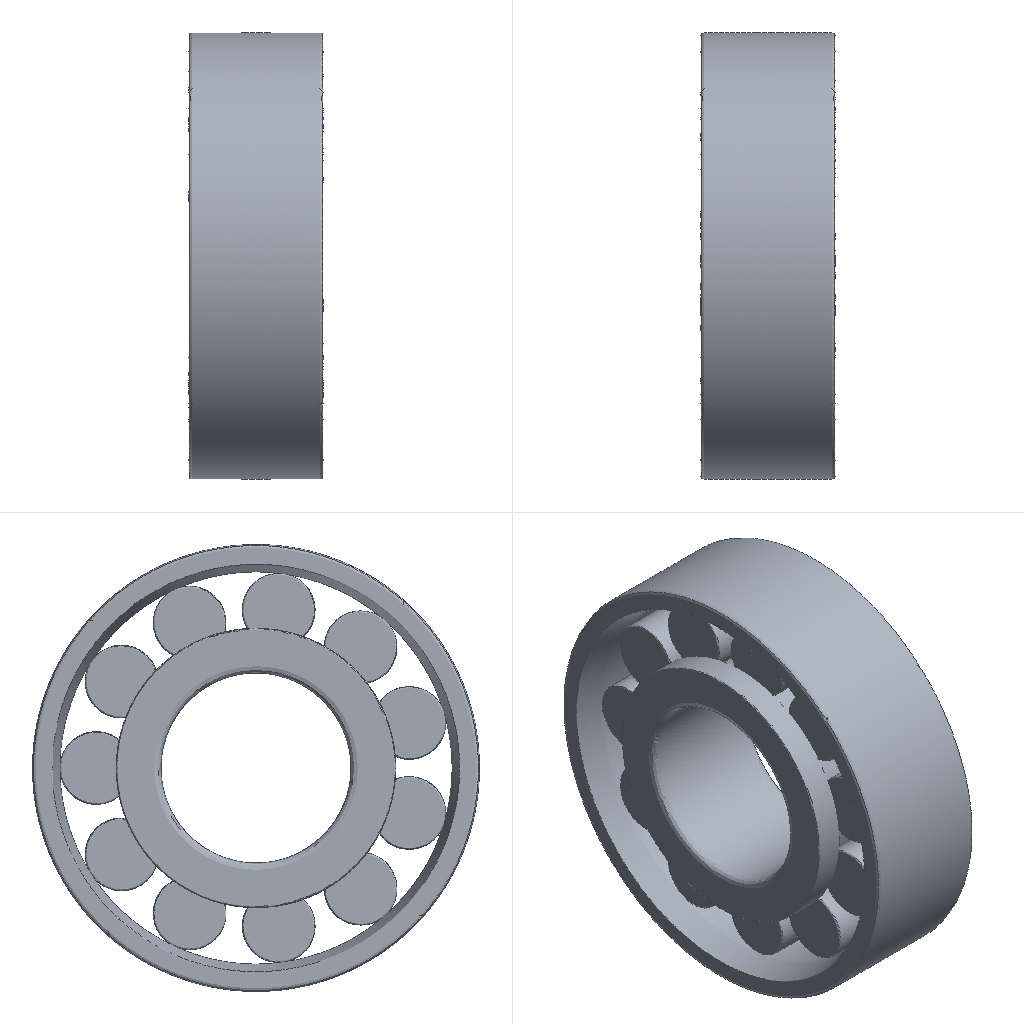Simulation study | ansys workbench
Set-up summary:
category,name,step,type,value,unit,region
solver,ansys_workbench
units,mm-N-s-tonne (MPa),,stated,"/units,MPA"
analysis,LS1,,static
load_step,LS1,LS1,static,nsubst=1; time=1
mesh,nodes,,,877286
mesh,elements,,,641316
element_type,SOLID187,,,594392
element_type,TARGE170,,,16923
element_type,CONTA174,,,16923
element_type,SURF154,,,13078
material,Structural Steel,,E,200000,tonne s^-2 mm^-1
material,Structural Steel,,nu,0.3
material,Structural Steel,,density,7.85e-09,tonne mm^-3
material,Structural Steel,,conductivity,60.5,tonne mm s^-3 C^-1
material,Structural Steel,,specific_heat,4.34e+08,mm^2 s^-2 C^-1
material,Structural Steel,,cte,1.2e-05,C^-1
material,Structural Steel,,permeability,10000
material,Structural Steel,,resistivity,0.00017,ohm mm
load,Define Force Using Surface Effect Elements,LS1,surface-effect pres face 2,-0.349,,SURF154 #8
bc,Constant Zero Displacement X,model,fixed,[dofs=UX],,_DISPZEROUX
bc,Constant Zero Displacement Y,model,fixed,[dofs=UY],,_DISPZEROUY
bc,Constant Zero Displacement Z,model,fixed,[dofs=UZ],,_DISPZEROUZ
contact,Contact Region,,bonded (always),element=CONTA174
contact,Contact Region 2,,bonded (always),element=CONTA174
named_set,_DISPZEROUX,,node,26660
named_set,_DISPZEROUY,,node,26660
named_set,_DISPZEROUZ,,node,26660
Ansys APDL input file, long lists of numbers shortened:
/batch
/config,noeldb,1     ! force off writing results to database
*get,_wallstrt,active,,time,wall
! ANSYS input file written by Workbench version 2022 R2
! File used for geometry attach:
/title,____--____ (A5)
! ****** Begin Custom Load Command Snippet ******
/COM, ACT Extensions:
/COM,     LSDYNA, 2022.2
/COM,/COM,     ANSYSMotion, 2022.2
/COM,
! ****** End   Custom Load Command Snippet ******
*DIM,_wb_ProjectScratch_dir,string,248
_wb_ProjectScratch_dir(1) = ''
*DIM,_wb_SolverFiles_dir,string,248
_wb_SolverFiles_dir(1) = ''
*DIM,_wb_userfiles_dir,string,248
_wb_userfiles_dir(1) = ''
/com,--- Data in consistent NMM units. See Solving Units in the help system for more information.
/units,MPA
/nopr
/wb,file,start              !  signify a WB generated input file
/prep7
! Turn off shape checking because checks already performed inside WB mesher.
! See help system for more information.
SHPP,OFF,,NOWARN
/nolist
etcon,set             ! allow ANSYS to choose best KEYOP's for 180x elements, resets any applicable keyopt to MAPDL defaults
/com,*********** Nodes for the whole assembly ***********
nblock,3,,965014
(1i9,3e20.9e3)
        1     6.000000000E-01     8.500000000E+00     0.000000000E+00
! (877285 more lines like these left out)
-1
/wb,elem,start            !  set before creation of elements
/com,*********** Elements for Body 1 "skf_bearing_n_203_ecp_2_1" ***********
et,1,187
eblock,19,solid,,168754
(19i9)
        1        1        1        1        0        0        0        0       10        0        1    24241    33706    28817    28794   205578   234077   205576   205574
! (337507 more lines like these left out)
-1
/com,*********** Elements for Body 2 "skf_bearing_n_203_ecp_2_2" ***********
et,2,187
eblock,19,solid,,244984
(19i9)
        2        2        2        2        0        0        0        0       10        0   349409   532471   543456   562473   549157   703456   779981   703461   703457
! (489967 more lines like these left out)
-1
/com,*********** Elements for Body 3 "skf_bearing_n_203_ecp_2_3" ***********
et,3,187
eblock,19,solid,,180654
(19i9)
        3        3        3        3        0        0        0        0       10        0   168755   276452   283271   278432   279668   480271   491944   480267   480268
! (361307 more lines like these left out)
-1
/wb,elem,end               !  done creating elements
/com,*********** Send User Defined Coordinate System(s) ***********
csys,0
toffst,273.15,  ! Temperature offset from absolute zero
/com,*********** Set Reference Temperature ***********
tref,22.
/wb,mat,start              !  starting to send materials
/com,*********** Send Materials ***********
Temperature = 'TEMP' ! Temperature
MP,DENS,1,7.85e-09,	! tonne mm^-3
MP,ALPX,1,1.2e-05,	! C^-1
MP,C,1,434000000,	! mm^2 s^-2 C^-1
MP,KXX,1,60.5,	! tonne mm s^-3 C^-1
MP,RSVX,1,0.00017,	! ohm mm
MP,EX,1,200000,	! tonne s^-2 mm^-1
MP,NUXY,1,0.3,
MP,MURX,1,10000,
Temperature = 'TEMP' ! Temperature
MP,DENS,2,7.85e-09,	! tonne mm^-3
MP,ALPX,2,1.2e-05,	! C^-1
MP,C,2,434000000,	! mm^2 s^-2 C^-1
MP,KXX,2,60.5,	! tonne mm s^-3 C^-1
MP,RSVX,2,0.00017,	! ohm mm
MP,EX,2,200000,	! tonne s^-2 mm^-1
MP,NUXY,2,0.3,
MP,MURX,2,10000,
Temperature = 'TEMP' ! Temperature
MP,DENS,3,7.85e-09,	! tonne mm^-3
MP,ALPX,3,1.2e-05,	! C^-1
MP,C,3,434000000,	! mm^2 s^-2 C^-1
MP,KXX,3,60.5,	! tonne mm s^-3 C^-1
MP,RSVX,3,0.00017,	! ohm mm
MP,EX,3,200000,	! tonne s^-2 mm^-1
MP,NUXY,3,0.3,
MP,MURX,3,10000,
/wb,mat,end                !  done sending materials
!************************* Model Summary ********************
!skf_bearing_n_203_ecp_2_1,	结构钢,	matid,	1
!skf_bearing_n_203_ecp_2_2,	结构钢,	matid,	2
!skf_bearing_n_203_ecp_2_3,	结构钢,	matid,	3
!************************* End Model Summary ********************
! get the diagonal of the bounding box. Needed later for other things
*get,_xmin,node,,mnloc,x
*get,_ymin,node,,mnloc,y
*get,_zmin,node,,mnloc,z
*get,_xmax,node,,mxloc,x
*get,_ymax,node,,mxloc,y
*get,_zmax,node,,mxloc,z
_ASMDIAG=(_xmax-_xmin)*(_xmax-_xmin)+(_ymax-_ymin)*(_ymax-_ymin)+(_zmax-_zmin)*(_zmax-_zmin)
_ASMDIAG=SQRT(_ASMDIAG)
/wb,contact,start          !  starting to send contact
/com,*********** Create Contact "接触区域" ***********
/com,            Real Constant Set For Above Contact Is 5 & 4
*set,tid,5
*set,cid,4
r,tid
r,cid
et,tid,170
et,cid,174
eblock,10,,,4315
(15i9)
   675971        5        5        5        0     8715     8859     8791     8791    93916    94399     8791    93915
! (4314 more lines like these left out)
-1
eblock,10,,,4315
(15i9)
   680286        4        4        4        0     8715     8859     8791     8791    93916    94399     8791    93915
! (4314 more lines like these left out)
-1
eblock,10,,,5558
(15i9)
   684601        4        5        4        0   258107   258138   258199   258199   357645   357931   258199   357648
! (5557 more lines like these left out)
-1
eblock,10,,,5558
(15i9)
   690159        5        4        5        0   258107   258138   258199   258199   357645   357931   258199   357648
! (5557 more lines like these left out)
-1
keyo,cid,8,2               ! auto create asymmetric contact (from Program Controlled setting)
keyo,cid,10,0              ! adjust contact stiffness each NR iteration (from Program Controlled setting)
keyo,cid,12,5              ! bonded always
keyo,cid,18,1              ! small sliding turned on by application
keyo,cid,2,0               ! augmented Lagrange (from Program Controlled setting)
keyo,cid,4,0               ! on Gauss point (from Program Controlled setting)
keyo,cid,9,1               ! ignore initial gaps/penetration
keyo,cid,7,0               ! No Prediction
rmod,tid,3,10.      ! FKN
rmod,tid,5,0.       ! ICONT
rmod,tid,6,0.       ! PINB
rmod,tid,10,0.      ! CNOF
rmod,tid,12,0.      ! FKT
rmod,tid,36,32      ! WB DSID
rmod,cid,3,10.      ! FKN
rmod,cid,5,0.       ! ICONT
rmod,cid,6,0.       ! PINB
rmod,cid,10,0.      ! CNOF
rmod,cid,12,0.      ! FKT
rmod,cid,36,32      ! WB DSID
/com,*********** Create Contact "接触区域 2" ***********
/com,            Real Constant Set For Above Contact Is 7 & 6
*set,tid,7
*set,cid,6
r,tid
r,cid
et,tid,170
et,cid,174
eblock,10,,,3223
(15i9)
   695717        7        7        7        0   512910   513130   519477   519477   571635   573570   519477   571638
! (3222 more lines like these left out)
-1
eblock,10,,,3223
(15i9)
   698940        6        6        6        0   512910   513130   519477   519477   571635   573570   519477   571638
! (3222 more lines like these left out)
-1
eblock,10,,,3827
(15i9)
   702163        6        7        6        0   246843   246842   249430   249430   283277   283280   249430   283288
! (3826 more lines like these left out)
-1
eblock,10,,,3827
(15i9)
   705990        7        6        7        0   246843   246842   249430   249430   283277   283280   249430   283288
! (3826 more lines like these left out)
-1
keyo,cid,8,2               ! auto create asymmetric contact (from Program Controlled setting)
keyo,cid,10,0              ! adjust contact stiffness each NR iteration (from Program Controlled setting)
keyo,cid,12,5              ! bonded always
keyo,cid,18,1              ! small sliding turned on by application
keyo,cid,2,0               ! augmented Lagrange (from Program Controlled setting)
keyo,cid,4,0               ! on Gauss point (from Program Controlled setting)
keyo,cid,9,1               ! ignore initial gaps/penetration
keyo,cid,7,0               ! No Prediction
rmod,tid,3,10.      ! FKN
rmod,tid,5,0.       ! ICONT
rmod,tid,6,0.       ! PINB
rmod,tid,10,0.      ! CNOF
rmod,tid,12,0.      ! FKT
rmod,tid,36,35      ! WB DSID
rmod,cid,3,10.      ! FKN
rmod,cid,5,0.       ! ICONT
rmod,cid,6,0.       ! PINB
rmod,cid,10,0.      ! CNOF
rmod,cid,12,0.      ! FKT
rmod,cid,36,35      ! WB DSID
nsel,all
esel,all
/wb,contact,end            !  done creating contacts
/golist
/wb,load,start             !  starting to send loads
/com,******* Constant Zero Displacement X *******
CMBLOCK,_DISPZEROUX,NODE,    26660
(8i10)
    511700    511701    511702    511703    511704    511705    511706    511707
! (3332 more lines like these left out)
cmsel,s,_DISPZEROUX
d,all,ux,0
nsel,all
/com,******* Constant Zero Displacement Y *******
CMBLOCK,_DISPZEROUY,NODE,    26660
(8i10)
    511700    511701    511702    511703    511704    511705    511706    511707
! (3332 more lines like these left out)
cmsel,s,_DISPZEROUY
d,all,uy,0
nsel,all
/com,******* Constant Zero Displacement Z *******
CMBLOCK,_DISPZEROUZ,NODE,    26660
(8i10)
    511700    511701    511702    511703    511704    511705    511706    511707
! (3332 more lines like these left out)
cmsel,s,_DISPZEROUZ
d,all,uz,0
nsel,all
/com,*********** Define Force Using Surface Effect Elements ***********
local,12,0,0.,0.,0.,0.,0.,0.
csys,0
et,8,154
eblock,10,,,13078
(15i9)
   709817        8        8        8       12   511959   511958   522804   522804   564554   564557   522804   564565
! (13077 more lines like these left out)
-1
esel,s,type,,8
keyop,8,2,1                ! Apply load in local coordinate system
keyop,8,7,1                ! Use original area so load is constant in large deformation
esel,all
/com,*********** Define Rotational Velocity ***********
esel,none
esel,a,type,,1
cm,cm_rotvelcity50,elem
esel,all
/gst,on,on
fini
*get,_numnode,node,0,count
*get,_numelem,elem,0,count
*get, _MAXELEMNUM, elem, 0, NUM, MAX
*get, _MAXNODENUM, node, 0, NUM, MAX
*get, _MAXELEMTYPE, etyp, 0, NUM, MAX
*get, _MAXREALCONST, rcon, 0, NUM, MAX
/go
/wb,load,end               !  done creating loads
/com,--- Number of total nodes = %_numnode%
/com,--- Number of contact elements = 46924
/com,--- Number of spring elements = 0
/com,--- Number of bearing elements = 0
/com,--- Number of solid elements = 594392
/com,--- Number of condensed parts = 0
/com,--- Number of total elements = %_numelem%
*get,_wallbsol,active,,time,wall
/com,****************************************************************************
/com,*************************    SOLUTION       ********************************
/com,****************************************************************************
/solu
antype,0                   ! static analysis
_thickRatio=  1     ! Ratio of thick parts in the model
eqsl,pcg,1e-8,,,,,,1
cntr,print,1               ! print out contact info and also make no initial contact an error
dmpoption,emat,no             ! Don't combine emat file for DANSYS
dmpoption,esav,no             ! Don't combine esav file for DANSYS
nldiag,cont,iter           ! print out contact info each equilibrium iteration
rescontrol,,none                 ! Do not keep any restart files
/com,****************************************************
/com,******************* SOLVE FOR LS 1 OF 1 ****************
esel,s,type,,8
nsle
sfe,all,1,pres,1,0.
sfe,all,2,pres,1,-0.349
sfe,all,3,pres,1,0.
nsel,all
esel,all
cmom,cm_rotvelcity50,200.,0.,0.,6.,0.,0.
/nopr
/gopr
nsub,1,1,1
time,1.
outres,erase
outres,all,none
outres,nsol,all,
outres,rsol,all
outres,eangl,all
outres,etmp,all
outres,veng,all
outres,strs,all,
outres,epel,all,
outres,eppl,all,
outres,cont,all,
! *********** WB SOLVE COMMAND ***********
! check interactive state
*get,ANSINTER_,active,,int
*if,ANSINTER_,ne,0,then
/eof
*endif
solve
/com *************** Write FE CONNECTORS *********
CEWRITE,file,ce,,INTE
/com,****************************************************
/com,*************** FINISHED SOLVE FOR LS 1 *************
*get,_wallasol,active,,time,wall
/nopr
*get,_numnode,node,0,count
*get,_numelem,elem,0,count
*get, _MAXELEMNUM, elem, 0, NUM, MAX
*get, _MAXNODENUM, node, 0, NUM, MAX,,,INTERNAL
*get, _MAXELEMTYPE, etyp, 0, NUM, MAX
*get, _MAXREALCONST, rcon, 0, NUM, MAX
*get,_NSOLTHREADS,active,0,ntfs
*get,_NSOLPROCESSES,active,0,npfs
/gopr
*get,_PCGITER,active,,solu,cgiter
/post1
xmlo,ENCODING,ISO-8859-1
xmlo,parm
/xml,parm,xml
fini
/gopr
*get,_walldone,active,,time,wall
_preptime=(_wallbsol-_wallstrt)*3600
_solvtime=(_wallasol-_wallbsol)*3600
_posttime=(_walldone-_wallasol)*3600
_totaltim=(_walldone-_wallstrt)*3600
*get,_dlbratio,active,0,solu,dlbr
*get,_combtime,active,0,solu,comb
*get,_ssmode,active,0,solu,ssmm
*get,_ndofs,active,0,solu,ndof
*get,_sol_end_time,active,0,set,time
*if,_sol_end_time,eq,1.,then
/fclean				!clean distributed files
*endif
/com,--- Total number of nodes = %_numnode%
/com,--- Total number of elements = %_numelem%
/com,--- Element load balance ratio = %_dlbratio%
/com,--- Time to combine distributed files = %_combtime%
/com,--- Sparse memory mode = %_ssmode%
/com,--- Number of DOF = %_ndofs%
/wb,file,end               ! done with WB generated input
Results summary:
result,analyses[0].index,,,1
result,analyses[0].system,,,SYS
result,analyses[0].deck,,,deck.dat
result,analyses[0].solve_status,,,completed
result,analyses[0].analysis_type,,,static
result,analyses[0].physics,,,mechanical
result,analyses[0].unit_system,,,"NMM: mm, ton, N, s, mV, mA, degC"
result,analyses[0].n_sets,,,1
result,analyses[0].load_steps[0].set,set=1,,1
result,analyses[0].load_steps[0].time_or_freq,set=1,,1
result,analyses[0].load_steps[0].max_displacement_magnitude,set=1,,9.90119e-07
result,analyses[0].load_steps[0].max_von_mises_nodal,set=1,,0.2984
result,analyses[0].load_steps[0].reaction_force_sum_xyz[1],set=1,,-7.57167e-11
result,analyses[0].load_steps[0].reaction_force_sum_xyz[2],set=1,,500
result,analyses[0].load_steps[0].reaction_force_sum_xyz[3],set=1,,-9.74449e-07